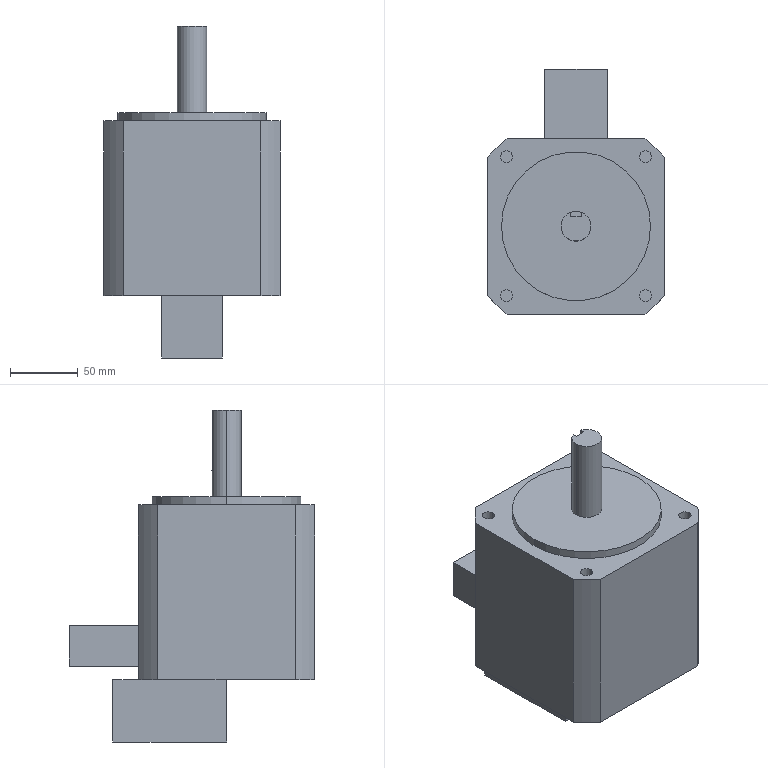Part | SolidWorks | features ICE 7, CirPattern 1, Extrusion 1, HoleWzd 1 | 1 solid | 43 faces | box 130 x 181 x 245 mm | volume 2453559 mm3 | plane 27 | cylinder 16 | commonest cylinder face diameters 9 x8 165 x4 22 x2 110 x2
STEP:
#1=CARTESIAN_POINT('',(46.765,51.265,0.));
#2=VERTEX_POINT('',#1);
#3=CARTESIAN_POINT('',(55.765,51.265,0.));
#4=VERTEX_POINT('',#3);
#5=CARTESIAN_POINT('',(51.265,51.265,0.));
#6=DIRECTION('',(0.,0.,1.));
#7=DIRECTION('',(1.,0.,0.));
#8=AXIS2_PLACEMENT_3D('',#5,#6,#7);
#9=CIRCLE('',#8,4.5);
#10=EDGE_CURVE('',#2,#4,#9,.T.);
#11=ORIENTED_EDGE('',*,*,#10,.F.);
#12=CARTESIAN_POINT('',(46.765,51.265,12.));
#13=VERTEX_POINT('',#12);
#14=CARTESIAN_POINT('',(46.765,51.265,12.));
#15=DIRECTION('',(0.,0.,1.));
#16=VECTOR('',#15,1000.);
#17=LINE('',#14,#16);
#18=EDGE_CURVE('',#2,#13,#17,.T.);
#19=ORIENTED_EDGE('',*,*,#18,.T.);
#20=CARTESIAN_POINT('',(55.765,51.265,12.));
#21=VERTEX_POINT('',#20);
#22=CARTESIAN_POINT('',(51.265,51.265,12.));
#23=DIRECTION('',(0.,0.,1.));
#24=DIRECTION('',(1.,0.,0.));
#25=AXIS2_PLACEMENT_3D('',#22,#23,#24);
#26=CIRCLE('',#25,4.5);
#27=EDGE_CURVE('',#13,#21,#26,.T.);
#28=ORIENTED_EDGE('',*,*,#27,.T.);
#29=CARTESIAN_POINT('',(55.765,51.265,12.));
#30=DIRECTION('',(0.,0.,1.));
#31=VECTOR('',#30,1000.);
#32=LINE('',#29,#31);
#33=EDGE_CURVE('',#4,#21,#32,.T.);
#34=ORIENTED_EDGE('',*,*,#33,.F.);
#35=EDGE_LOOP('',(#11,#19,#28,#34));
#36=FACE_OUTER_BOUND('',#35,.T.);
#37=CARTESIAN_POINT('',(51.265,51.265,12.));
#38=DIRECTION('',(0.,0.,1.));
#39=DIRECTION('',(1.,0.,0.));
#40=AXIS2_PLACEMENT_3D('',#37,#38,#39);
#41=CYLINDRICAL_SURFACE('',#40,4.5);
#42=ADVANCED_FACE('',(#36),#41,.F.);
#43=CARTESIAN_POINT('',(46.765,-51.265,0.));
#44=VERTEX_POINT('',#43);
#45=CARTESIAN_POINT('',(55.765,-51.265,0.));
#46=VERTEX_POINT('',#45);
#47=CARTESIAN_POINT('',(51.265,-51.265,0.));
#48=DIRECTION('',(0.,0.,1.));
#49=DIRECTION('',(1.,0.,0.));
#50=AXIS2_PLACEMENT_3D('',#47,#48,#49);
#51=CIRCLE('',#50,4.5);
#52=EDGE_CURVE('',#44,#46,#51,.T.);
#53=ORIENTED_EDGE('',*,*,#52,.F.);
#54=CARTESIAN_POINT('',(46.765,-51.265,12.));
#55=VERTEX_POINT('',#54);
#56=CARTESIAN_POINT('',(46.765,-51.265,12.));
#57=DIRECTION('',(0.,0.,1.));
#58=VECTOR('',#57,1000.);
#59=LINE('',#56,#58);
#60=EDGE_CURVE('',#44,#55,#59,.T.);
#61=ORIENTED_EDGE('',*,*,#60,.T.);
#62=CARTESIAN_POINT('',(55.765,-51.265,12.));
#63=VERTEX_POINT('',#62);
#64=CARTESIAN_POINT('',(51.265,-51.265,12.));
#65=DIRECTION('',(0.,0.,1.));
#66=DIRECTION('',(1.,0.,0.));
#67=AXIS2_PLACEMENT_3D('',#64,#65,#66);
#68=CIRCLE('',#67,4.5);
#69=EDGE_CURVE('',#55,#63,#68,.T.);
#70=ORIENTED_EDGE('',*,*,#69,.T.);
#71=CARTESIAN_POINT('',(55.765,-51.265,12.));
#72=DIRECTION('',(0.,0.,1.));
#73=VECTOR('',#72,1000.);
#74=LINE('',#71,#73);
#75=EDGE_CURVE('',#46,#63,#74,.T.);
#76=ORIENTED_EDGE('',*,*,#75,.F.);
#77=EDGE_LOOP('',(#53,#61,#70,#76));
#78=FACE_OUTER_BOUND('',#77,.T.);
#79=CARTESIAN_POINT('',(51.265,-51.265,12.));
#80=DIRECTION('',(0.,0.,1.));
#81=DIRECTION('',(1.,0.,0.));
#82=AXIS2_PLACEMENT_3D('',#79,#80,#81);
#83=CYLINDRICAL_SURFACE('',#82,4.5);
#84=ADVANCED_FACE('',(#78),#83,.F.);
#85=CARTESIAN_POINT('',(-55.765,-51.265,0.));
#86=VERTEX_POINT('',#85);
#87=CARTESIAN_POINT('',(-46.765,-51.265,0.));
#88=VERTEX_POINT('',#87);
#89=CARTESIAN_POINT('',(-51.265,-51.265,0.));
#90=DIRECTION('',(0.,0.,1.));
#91=DIRECTION('',(1.,0.,0.));
#92=AXIS2_PLACEMENT_3D('',#89,#90,#91);
#93=CIRCLE('',#92,4.5);
#94=EDGE_CURVE('',#86,#88,#93,.T.);
#95=ORIENTED_EDGE('',*,*,#94,.F.);
#96=CARTESIAN_POINT('',(-55.765,-51.265,12.));
#97=VERTEX_POINT('',#96);
#98=CARTESIAN_POINT('',(-55.765,-51.265,12.));
#99=DIRECTION('',(0.,0.,1.));
#100=VECTOR('',#99,1000.);
#101=LINE('',#98,#100);
#102=EDGE_CURVE('',#86,#97,#101,.T.);
#103=ORIENTED_EDGE('',*,*,#102,.T.);
#104=CARTESIAN_POINT('',(-46.765,-51.265,12.));
#105=VERTEX_POINT('',#104);
#106=CARTESIAN_POINT('',(-51.265,-51.265,12.));
#107=DIRECTION('',(0.,0.,1.));
#108=DIRECTION('',(1.,0.,0.));
#109=AXIS2_PLACEMENT_3D('',#106,#107,#108);
#110=CIRCLE('',#109,4.5);
#111=EDGE_CURVE('',#97,#105,#110,.T.);
#112=ORIENTED_EDGE('',*,*,#111,.T.);
#113=CARTESIAN_POINT('',(-46.765,-51.265,12.));
#114=DIRECTION('',(0.,0.,1.));
#115=VECTOR('',#114,1000.);
#116=LINE('',#113,#115);
#117=EDGE_CURVE('',#88,#105,#116,.T.);
#118=ORIENTED_EDGE('',*,*,#117,.F.);
#119=EDGE_LOOP('',(#95,#103,#112,#118));
#120=FACE_OUTER_BOUND('',#119,.T.);
#121=CARTESIAN_POINT('',(-51.265,-51.265,12.));
#122=DIRECTION('',(0.,0.,1.));
#123=DIRECTION('',(1.,0.,0.));
#124=AXIS2_PLACEMENT_3D('',#121,#122,#123);
#125=CYLINDRICAL_SURFACE('',#124,4.5);
#126=ADVANCED_FACE('',(#120),#125,.F.);
#127=CARTESIAN_POINT('',(-55.765,51.265,0.));
#128=VERTEX_POINT('',#127);
#129=CARTESIAN_POINT('',(-46.765,51.265,0.));
#130=VERTEX_POINT('',#129);
#131=CARTESIAN_POINT('',(-51.265,51.265,0.));
#132=DIRECTION('',(0.,0.,1.));
#133=DIRECTION('',(1.,0.,0.));
#134=AXIS2_PLACEMENT_3D('',#131,#132,#133);
#135=CIRCLE('',#134,4.5);
#136=EDGE_CURVE('',#128,#130,#135,.T.);
#137=ORIENTED_EDGE('',*,*,#136,.F.);
#138=CARTESIAN_POINT('',(-55.765,51.265,12.));
#139=VERTEX_POINT('',#138);
#140=CARTESIAN_POINT('',(-55.765,51.265,12.));
#141=DIRECTION('',(0.,0.,1.));
#142=VECTOR('',#141,1000.);
#143=LINE('',#140,#142);
#144=EDGE_CURVE('',#128,#139,#143,.T.);
#145=ORIENTED_EDGE('',*,*,#144,.T.);
#146=CARTESIAN_POINT('',(-46.765,51.265,12.));
#147=VERTEX_POINT('',#146);
#148=CARTESIAN_POINT('',(-51.265,51.265,12.));
#149=DIRECTION('',(0.,0.,1.));
#150=DIRECTION('',(1.,0.,0.));
#151=AXIS2_PLACEMENT_3D('',#148,#149,#150);
#152=CIRCLE('',#151,4.5);
#153=EDGE_CURVE('',#139,#147,#152,.T.);
#154=ORIENTED_EDGE('',*,*,#153,.T.);
#155=CARTESIAN_POINT('',(-46.765,51.265,12.));
#156=DIRECTION('',(0.,0.,1.));
#157=VECTOR('',#156,1000.);
#158=LINE('',#155,#157);
#159=EDGE_CURVE('',#130,#147,#158,.T.);
#160=ORIENTED_EDGE('',*,*,#159,.F.);
#161=EDGE_LOOP('',(#137,#145,#154,#160));
#162=FACE_OUTER_BOUND('',#161,.T.);
#163=CARTESIAN_POINT('',(-51.265,51.265,12.));
#164=DIRECTION('',(0.,0.,1.));
#165=DIRECTION('',(1.,0.,0.));
#166=AXIS2_PLACEMENT_3D('',#163,#164,#165);
#167=CYLINDRICAL_SURFACE('',#166,4.5);
#168=ADVANCED_FACE('',(#162),#167,.F.);
#169=CARTESIAN_POINT('',(11.,0.,82.));
#170=VERTEX_POINT('',#169);
#171=CARTESIAN_POINT('',(4.,10.247,82.));
#172=VERTEX_POINT('',#171);
#173=CARTESIAN_POINT('',(0.,0.,82.));
#174=DIRECTION('',(0.,0.,1.));
#175=DIRECTION('',(1.,0.,0.));
#176=AXIS2_PLACEMENT_3D('',#173,#174,#175);
#177=CIRCLE('',#176,11.);
#178=EDGE_CURVE('',#170,#172,#177,.T.);
#179=ORIENTED_EDGE('',*,*,#178,.F.);
#180=CARTESIAN_POINT('',(11.,0.,18.));
#181=VERTEX_POINT('',#180);
#182=CARTESIAN_POINT('',(11.,0.,82.));
#183=DIRECTION('',(0.,0.,-1.));
#184=VECTOR('',#183,1000.);
#185=LINE('',#182,#184);
#186=EDGE_CURVE('',#170,#181,#185,.T.);
#187=ORIENTED_EDGE('',*,*,#186,.T.);
#188=CARTESIAN_POINT('',(-11.,0.,18.));
#189=VERTEX_POINT('',#188);
#190=CARTESIAN_POINT('',(0.,0.,18.));
#191=DIRECTION('',(0.,0.,1.));
#192=DIRECTION('',(1.,0.,0.));
#193=AXIS2_PLACEMENT_3D('',#190,#191,#192);
#194=CIRCLE('',#193,11.);
#195=EDGE_CURVE('',#181,#189,#194,.T.);
#196=ORIENTED_EDGE('',*,*,#195,.T.);
#197=CARTESIAN_POINT('',(-11.,0.,82.));
#198=VERTEX_POINT('',#197);
#199=CARTESIAN_POINT('',(-11.,0.,82.));
#200=DIRECTION('',(0.,0.,-1.));
#201=VECTOR('',#200,1000.);
#202=LINE('',#199,#201);
#203=EDGE_CURVE('',#198,#189,#202,.T.);
#204=ORIENTED_EDGE('',*,*,#203,.F.);
#205=CARTESIAN_POINT('',(-4.,10.247,82.));
#206=VERTEX_POINT('',#205);
#207=CARTESIAN_POINT('',(0.,0.,82.));
#208=DIRECTION('',(0.,0.,1.));
#209=DIRECTION('',(1.,0.,0.));
#210=AXIS2_PLACEMENT_3D('',#207,#208,#209);
#211=CIRCLE('',#210,11.);
#212=EDGE_CURVE('',#206,#198,#211,.T.);
#213=ORIENTED_EDGE('',*,*,#212,.F.);
#214=CARTESIAN_POINT('',(-4.,10.247,37.));
#215=VERTEX_POINT('',#214);
#216=CARTESIAN_POINT('',(-4.,10.247,82.));
#217=DIRECTION('',(0.,0.,-1.));
#218=VECTOR('',#217,1000.);
#219=LINE('',#216,#218);
#220=EDGE_CURVE('',#206,#215,#219,.T.);
#221=ORIENTED_EDGE('',*,*,#220,.T.);
#222=CARTESIAN_POINT('',(4.,10.247,37.));
#223=VERTEX_POINT('',#222);
#224=CARTESIAN_POINT('',(0.,0.,37.));
#225=DIRECTION('',(0.,0.,-1.));
#226=DIRECTION('',(-1.,0.,0.));
#227=AXIS2_PLACEMENT_3D('',#224,#225,#226);
#228=CIRCLE('',#227,11.);
#229=EDGE_CURVE('',#215,#223,#228,.T.);
#230=ORIENTED_EDGE('',*,*,#229,.T.);
#231=CARTESIAN_POINT('',(4.,10.247,82.));
#232=DIRECTION('',(0.,0.,1.));
#233=VECTOR('',#232,1000.);
#234=LINE('',#231,#233);
#235=EDGE_CURVE('',#223,#172,#234,.T.);
#236=ORIENTED_EDGE('',*,*,#235,.T.);
#237=EDGE_LOOP('',(#179,#187,#196,#204,#213,#221,#230,#236));
#238=FACE_OUTER_BOUND('',#237,.T.);
#239=CARTESIAN_POINT('',(0.,0.,82.));
#240=DIRECTION('',(0.,0.,-1.));
#241=DIRECTION('',(-1.,0.,0.));
#242=AXIS2_PLACEMENT_3D('',#239,#240,#241);
#243=CYLINDRICAL_SURFACE('',#242,11.);
#244=ADVANCED_FACE('',(#238),#243,.T.);
#245=CARTESIAN_POINT('',(55.,0.,18.));
#246=VERTEX_POINT('',#245);
#247=CARTESIAN_POINT('',(-55.,0.,18.));
#248=VERTEX_POINT('',#247);
#249=CARTESIAN_POINT('',(0.,0.,18.));
#250=DIRECTION('',(0.,0.,1.));
#251=DIRECTION('',(1.,0.,0.));
#252=AXIS2_PLACEMENT_3D('',#249,#250,#251);
#253=CIRCLE('',#252,55.);
#254=EDGE_CURVE('',#246,#248,#253,.T.);
#255=ORIENTED_EDGE('',*,*,#254,.F.);
#256=CARTESIAN_POINT('',(55.,0.,12.));
#257=VERTEX_POINT('',#256);
#258=CARTESIAN_POINT('',(55.,0.,18.));
#259=DIRECTION('',(0.,0.,-1.));
#260=VECTOR('',#259,1000.);
#261=LINE('',#258,#260);
#262=EDGE_CURVE('',#246,#257,#261,.T.);
#263=ORIENTED_EDGE('',*,*,#262,.T.);
#264=CARTESIAN_POINT('',(-55.,0.,12.));
#265=VERTEX_POINT('',#264);
#266=CARTESIAN_POINT('',(0.,0.,12.));
#267=DIRECTION('',(0.,0.,1.));
#268=DIRECTION('',(1.,0.,0.));
#269=AXIS2_PLACEMENT_3D('',#266,#267,#268);
#270=CIRCLE('',#269,55.);
#271=EDGE_CURVE('',#257,#265,#270,.T.);
#272=ORIENTED_EDGE('',*,*,#271,.T.);
#273=CARTESIAN_POINT('',(-55.,0.,18.));
#274=DIRECTION('',(0.,0.,-1.));
#275=VECTOR('',#274,1000.);
#276=LINE('',#273,#275);
#277=EDGE_CURVE('',#248,#265,#276,.T.);
#278=ORIENTED_EDGE('',*,*,#277,.F.);
#279=EDGE_LOOP('',(#255,#263,#272,#278));
#280=FACE_OUTER_BOUND('',#279,.T.);
#281=CARTESIAN_POINT('',(0.,0.,18.));
#282=DIRECTION('',(0.,0.,-1.));
#283=DIRECTION('',(-1.,0.,0.));
#284=AXIS2_PLACEMENT_3D('',#281,#282,#283);
#285=CYLINDRICAL_SURFACE('',#284,55.);
#286=ADVANCED_FACE('',(#280),#285,.T.);
#287=CARTESIAN_POINT('',(51.265,51.265,12.));
#288=DIRECTION('',(0.,0.,1.));
#289=DIRECTION('',(1.,0.,0.));
#290=AXIS2_PLACEMENT_3D('',#287,#288,#289);
#291=CIRCLE('',#290,4.5);
#292=EDGE_CURVE('',#21,#13,#291,.T.);
#293=ORIENTED_EDGE('',*,*,#292,.F.);
#294=ORIENTED_EDGE('',*,*,#27,.F.);
#295=EDGE_LOOP('',(#293,#294));
#296=FACE_BOUND('',#295,.T.);
#297=CARTESIAN_POINT('',(51.265,-51.265,12.));
#298=DIRECTION('',(0.,0.,1.));
#299=DIRECTION('',(1.,0.,0.));
#300=AXIS2_PLACEMENT_3D('',#297,#298,#299);
#301=CIRCLE('',#300,4.5);
#302=EDGE_CURVE('',#63,#55,#301,.T.);
#303=ORIENTED_EDGE('',*,*,#302,.F.);
#304=ORIENTED_EDGE('',*,*,#69,.F.);
#305=EDGE_LOOP('',(#303,#304));
#306=FACE_BOUND('',#305,.T.);
#307=CARTESIAN_POINT('',(-51.265,-51.265,12.));
#308=DIRECTION('',(0.,0.,1.));
#309=DIRECTION('',(1.,0.,0.));
#310=AXIS2_PLACEMENT_3D('',#307,#308,#309);
#311=CIRCLE('',#310,4.5);
#312=EDGE_CURVE('',#105,#97,#311,.T.);
#313=ORIENTED_EDGE('',*,*,#312,.F.);
#314=ORIENTED_EDGE('',*,*,#111,.F.);
#315=EDGE_LOOP('',(#313,#314));
#316=FACE_BOUND('',#315,.T.);
#317=CARTESIAN_POINT('',(-51.265,51.265,12.));
#318=DIRECTION('',(0.,0.,1.));
#319=DIRECTION('',(1.,0.,0.));
#320=AXIS2_PLACEMENT_3D('',#317,#318,#319);
#321=CIRCLE('',#320,4.5);
#322=EDGE_CURVE('',#147,#139,#321,.T.);
#323=ORIENTED_EDGE('',*,*,#322,.F.);
#324=ORIENTED_EDGE('',*,*,#153,.F.);
#325=EDGE_LOOP('',(#323,#324));
#326=FACE_BOUND('',#325,.T.);
#327=CARTESIAN_POINT('',(0.,0.,12.));
#328=DIRECTION('',(0.,0.,1.));
#329=DIRECTION('',(1.,0.,0.));
#330=AXIS2_PLACEMENT_3D('',#327,#328,#329);
#331=CIRCLE('',#330,55.);
#332=EDGE_CURVE('',#265,#257,#331,.T.);
#333=ORIENTED_EDGE('',*,*,#332,.F.);
#334=ORIENTED_EDGE('',*,*,#271,.F.);
#335=EDGE_LOOP('',(#333,#334));
#336=FACE_BOUND('',#335,.T.);
#337=CARTESIAN_POINT('',(65.,-50.806,12.));
#338=VERTEX_POINT('',#337);
#339=CARTESIAN_POINT('',(65.,50.806,12.));
#340=VERTEX_POINT('',#339);
#341=CARTESIAN_POINT('',(65.,65.,12.));
#342=DIRECTION('',(0.,1.,0.));
#343=VECTOR('',#342,1000.);
#344=LINE('',#341,#343);
#345=EDGE_CURVE('',#338,#340,#344,.T.);
#346=ORIENTED_EDGE('',*,*,#345,.T.);
#347=CARTESIAN_POINT('',(50.806,65.,12.));
#348=VERTEX_POINT('',#347);
#349=CARTESIAN_POINT('',(0.,0.,12.));
#350=DIRECTION('',(0.,0.,1.));
#351=DIRECTION('',(1.,0.,0.));
#352=AXIS2_PLACEMENT_3D('',#349,#350,#351);
#353=CIRCLE('',#352,82.5);
#354=EDGE_CURVE('',#340,#348,#353,.T.);
#355=ORIENTED_EDGE('',*,*,#354,.T.);
#356=CARTESIAN_POINT('',(-50.806,65.,12.));
#357=VERTEX_POINT('',#356);
#358=CARTESIAN_POINT('',(-65.,65.,12.));
#359=DIRECTION('',(-1.,0.,0.));
#360=VECTOR('',#359,1000.);
#361=LINE('',#358,#360);
#362=EDGE_CURVE('',#348,#357,#361,.T.);
#363=ORIENTED_EDGE('',*,*,#362,.T.);
#364=CARTESIAN_POINT('',(-65.,50.806,12.));
#365=VERTEX_POINT('',#364);
#366=CARTESIAN_POINT('',(0.,0.,12.));
#367=DIRECTION('',(0.,0.,1.));
#368=DIRECTION('',(1.,0.,0.));
#369=AXIS2_PLACEMENT_3D('',#366,#367,#368);
#370=CIRCLE('',#369,82.5);
#371=EDGE_CURVE('',#357,#365,#370,.T.);
#372=ORIENTED_EDGE('',*,*,#371,.T.);
#373=CARTESIAN_POINT('',(-65.,-50.806,12.));
#374=VERTEX_POINT('',#373);
#375=CARTESIAN_POINT('',(-65.,65.,12.));
#376=DIRECTION('',(0.,-1.,0.));
#377=VECTOR('',#376,1000.);
#378=LINE('',#375,#377);
#379=EDGE_CURVE('',#365,#374,#378,.T.);
#380=ORIENTED_EDGE('',*,*,#379,.T.);
#381=CARTESIAN_POINT('',(-50.806,-65.,12.));
#382=VERTEX_POINT('',#381);
#383=CARTESIAN_POINT('',(0.,0.,12.));
#384=DIRECTION('',(0.,0.,1.));
#385=DIRECTION('',(1.,0.,0.));
#386=AXIS2_PLACEMENT_3D('',#383,#384,#385);
#387=CIRCLE('',#386,82.5);
#388=EDGE_CURVE('',#374,#382,#387,.T.);
#389=ORIENTED_EDGE('',*,*,#388,.T.);
#390=CARTESIAN_POINT('',(50.806,-65.,12.));
#391=VERTEX_POINT('',#390);
#392=CARTESIAN_POINT('',(-65.,-65.,12.));
#393=DIRECTION('',(1.,0.,0.));
#394=VECTOR('',#393,1000.);
#395=LINE('',#392,#394);
#396=EDGE_CURVE('',#382,#391,#395,.T.);
#397=ORIENTED_EDGE('',*,*,#396,.T.);
#398=CARTESIAN_POINT('',(0.,0.,12.));
#399=DIRECTION('',(0.,0.,1.));
#400=DIRECTION('',(1.,0.,0.));
#401=AXIS2_PLACEMENT_3D('',#398,#399,#400);
#402=CIRCLE('',#401,82.5);
#403=EDGE_CURVE('',#391,#338,#402,.T.);
#404=ORIENTED_EDGE('',*,*,#403,.T.);
#405=EDGE_LOOP('',(#346,#355,#363,#372,#380,#389,#397,#404));
#406=FACE_OUTER_BOUND('',#405,.T.);
#407=CARTESIAN_POINT('',(65.,-65.,12.));
#408=DIRECTION('',(0.,0.,1.));
#409=DIRECTION('',(1.,0.,0.));
#410=AXIS2_PLACEMENT_3D('',#407,#408,#409);
#411=PLANE('',#410);
#412=ADVANCED_FACE('',(#296,#306,#316,#326,#336,#406),#411,.T.);
#413=CARTESIAN_POINT('',(65.,-50.806,-117.));
#414=VERTEX_POINT('',#413);
#415=CARTESIAN_POINT('',(65.,-50.806,-52.));
#416=DIRECTION('',(0.,0.,1.));
#417=VECTOR('',#416,1000.);
#418=LINE('',#415,#417);
#419=EDGE_CURVE('',#414,#338,#418,.T.);
#420=ORIENTED_EDGE('',*,*,#419,.F.);
#421=CARTESIAN_POINT('',(65.,50.806,-117.));
#422=VERTEX_POINT('',#421);
#423=CARTESIAN_POINT('',(65.,50.806,-117.));
#424=DIRECTION('',(0.,-1.,0.));
#425=VECTOR('',#424,1000.);
#426=LINE('',#423,#425);
#427=EDGE_CURVE('',#422,#414,#426,.T.);
#428=ORIENTED_EDGE('',*,*,#427,.F.);
#429=CARTESIAN_POINT('',(65.,50.806,-52.));
#430=DIRECTION('',(0.,0.,-1.));
#431=VECTOR('',#430,1000.);
#432=LINE('',#429,#431);
#433=EDGE_CURVE('',#340,#422,#432,.T.);
#434=ORIENTED_EDGE('',*,*,#433,.F.);
#435=ORIENTED_EDGE('',*,*,#345,.F.);
#436=EDGE_LOOP('',(#420,#428,#434,#435));
#437=FACE_OUTER_BOUND('',#436,.T.);
#438=CARTESIAN_POINT('',(65.,65.,12.));
#439=DIRECTION('',(-1.,0.,0.));
#440=DIRECTION('',(0.,-1.,0.));
#441=AXIS2_PLACEMENT_3D('',#438,#439,#440);
#442=PLANE('',#441);
#443=ADVANCED_FACE('',(#437),#442,.F.);
#444=CARTESIAN_POINT('',(23.,65.,-107.));
#445=VERTEX_POINT('',#444);
#446=CARTESIAN_POINT('',(-23.,65.,-107.));
#447=VERTEX_POINT('',#446);
#448=CARTESIAN_POINT('',(23.,65.,-107.));
#449=DIRECTION('',(-1.,0.,0.));
#450=VECTOR('',#449,1000.);
#451=LINE('',#448,#450);
#452=EDGE_CURVE('',#445,#447,#451,.T.);
#453=ORIENTED_EDGE('',*,*,#452,.F.);
#454=CARTESIAN_POINT('',(23.,65.,-77.));
#455=VERTEX_POINT('',#454);
#456=CARTESIAN_POINT('',(23.,65.,-107.));
#457=DIRECTION('',(0.,0.,-1.));
#458=VECTOR('',#457,1000.);
#459=LINE('',#456,#458);
#460=EDGE_CURVE('',#455,#445,#459,.T.);
#461=ORIENTED_EDGE('',*,*,#460,.F.);
#462=CARTESIAN_POINT('',(-23.,65.,-77.));
#463=VERTEX_POINT('',#462);
#464=CARTESIAN_POINT('',(23.,65.,-77.));
#465=DIRECTION('',(-1.,0.,0.));
#466=VECTOR('',#465,1000.);
#467=LINE('',#464,#466);
#468=EDGE_CURVE('',#455,#463,#467,.T.);
#469=ORIENTED_EDGE('',*,*,#468,.T.);
#470=CARTESIAN_POINT('',(-23.,65.,-107.));
#471=DIRECTION('',(0.,0.,-1.));
#472=VECTOR('',#471,1000.);
#473=LINE('',#470,#472);
#474=EDGE_CURVE('',#463,#447,#473,.T.);
#475=ORIENTED_EDGE('',*,*,#474,.T.);
#476=EDGE_LOOP('',(#453,#461,#469,#475));
#477=FACE_BOUND('',#476,.T.);
#478=CARTESIAN_POINT('',(50.806,65.,-117.));
#479=VERTEX_POINT('',#478);
#480=CARTESIAN_POINT('',(50.806,65.,-52.));
#481=DIRECTION('',(0.,0.,1.));
#482=VECTOR('',#481,1000.);
#483=LINE('',#480,#482);
#484=EDGE_CURVE('',#479,#348,#483,.T.);
#485=ORIENTED_EDGE('',*,*,#484,.F.);
#486=CARTESIAN_POINT('',(22.5,65.,-117.));
#487=VERTEX_POINT('',#486);
#488=CARTESIAN_POINT('',(-50.806,65.,-117.));
#489=DIRECTION('',(1.,0.,0.));
#490=VECTOR('',#489,1000.);
#491=LINE('',#488,#490);
#492=EDGE_CURVE('',#487,#479,#491,.T.);
#493=ORIENTED_EDGE('',*,*,#492,.F.);
#494=CARTESIAN_POINT('',(-22.5,65.,-117.));
#495=VERTEX_POINT('',#494);
#496=CARTESIAN_POINT('',(-50.806,65.,-117.));
#497=DIRECTION('',(1.,0.,0.));
#498=VECTOR('',#497,1000.);
#499=LINE('',#496,#498);
#500=EDGE_CURVE('',#495,#487,#499,.T.);
#501=ORIENTED_EDGE('',*,*,#500,.F.);
#502=CARTESIAN_POINT('',(-50.806,65.,-117.));
#503=VERTEX_POINT('',#502);
#504=CARTESIAN_POINT('',(-50.806,65.,-117.));
#505=DIRECTION('',(1.,0.,0.));
#506=VECTOR('',#505,1000.);
#507=LINE('',#504,#506);
#508=EDGE_CURVE('',#503,#495,#507,.T.);
#509=ORIENTED_EDGE('',*,*,#508,.F.);
#510=CARTESIAN_POINT('',(-50.806,65.,-52.));
#511=DIRECTION('',(0.,0.,-1.));
#512=VECTOR('',#511,1000.);
#513=LINE('',#510,#512);
#514=EDGE_CURVE('',#357,#503,#513,.T.);
#515=ORIENTED_EDGE('',*,*,#514,.F.);
#516=ORIENTED_EDGE('',*,*,#362,.F.);
#517=EDGE_LOOP('',(#485,#493,#501,#509,#515,#516));
#518=FACE_OUTER_BOUND('',#517,.T.);
#519=CARTESIAN_POINT('',(-65.,65.,12.));
#520=DIRECTION('',(0.,-1.,0.));
#521=DIRECTION('',(0.,0.,-1.));
#522=AXIS2_PLACEMENT_3D('',#519,#520,#521);
#523=PLANE('',#522);
#524=ADVANCED_FACE('',(#477,#518),#523,.F.);
#525=CARTESIAN_POINT('',(-65.,50.806,-117.));
#526=VERTEX_POINT('',#525);
#527=CARTESIAN_POINT('',(-65.,50.806,-52.));
#528=DIRECTION('',(0.,0.,1.));
#529=VECTOR('',#528,1000.);
#530=LINE('',#527,#529);
#531=EDGE_CURVE('',#526,#365,#530,.T.);
#532=ORIENTED_EDGE('',*,*,#531,.F.);
#533=CARTESIAN_POINT('',(-65.,-50.806,-117.));
#534=VERTEX_POINT('',#533);
#535=CARTESIAN_POINT('',(-65.,-50.806,-117.));
#536=DIRECTION('',(0.,1.,0.));
#537=VECTOR('',#536,1000.);
#538=LINE('',#535,#537);
#539=EDGE_CURVE('',#534,#526,#538,.T.);
#540=ORIENTED_EDGE('',*,*,#539,.F.);
#541=CARTESIAN_POINT('',(-65.,-50.806,-52.));
#542=DIRECTION('',(0.,0.,-1.));
#543=VECTOR('',#542,1000.);
#544=LINE('',#541,#543);
#545=EDGE_CURVE('',#374,#534,#544,.T.);
#546=ORIENTED_EDGE('',*,*,#545,.F.);
#547=ORIENTED_EDGE('',*,*,#379,.F.);
#548=EDGE_LOOP('',(#532,#540,#546,#547));
#549=FACE_OUTER_BOUND('',#548,.T.);
#550=CARTESIAN_POINT('',(-65.,65.,12.));
#551=DIRECTION('',(1.,0.,0.));
#552=DIRECTION('',(0.,1.,0.));
#553=AXIS2_PLACEMENT_3D('',#550,#551,#552);
#554=PLANE('',#553);
#555=ADVANCED_FACE('',(#549),#554,.F.);
#556=CARTESIAN_POINT('',(-50.806,-65.,-117.));
#557=VERTEX_POINT('',#556);
#558=CARTESIAN_POINT('',(-50.806,-65.,-52.));
#559=DIRECTION('',(0.,0.,1.));
#560=VECTOR('',#559,1000.);
#561=LINE('',#558,#560);
#562=EDGE_CURVE('',#557,#382,#561,.T.);
#563=ORIENTED_EDGE('',*,*,#562,.F.);
#564=CARTESIAN_POINT('',(50.806,-65.,-117.));
#565=VERTEX_POINT('',#564);
#566=CARTESIAN_POINT('',(50.806,-65.,-117.));
#567=DIRECTION('',(-1.,0.,0.));
#568=VECTOR('',#567,1000.);
#569=LINE('',#566,#568);
#570=EDGE_CURVE('',#565,#557,#569,.T.);
#571=ORIENTED_EDGE('',*,*,#570,.F.);
#572=CARTESIAN_POINT('',(50.806,-65.,-52.));
#573=DIRECTION('',(0.,0.,-1.));
#574=VECTOR('',#573,1000.);
#575=LINE('',#572,#574);
#576=EDGE_CURVE('',#391,#565,#575,.T.);
#577=ORIENTED_EDGE('',*,*,#576,.F.);
#578=ORIENTED_EDGE('',*,*,#396,.F.);
#579=EDGE_LOOP('',(#563,#571,#577,#578));
#580=FACE_OUTER_BOUND('',#579,.T.);
#581=CARTESIAN_POINT('',(-65.,-65.,12.));
#582=DIRECTION('',(0.,1.,0.));
#583=DIRECTION('',(0.,0.,1.));
#584=AXIS2_PLACEMENT_3D('',#581,#582,#583);
#585=PLANE('',#584);
#586=ADVANCED_FACE('',(#580),#585,.F.);
#587=CARTESIAN_POINT('',(0.,0.,18.));
#588=DIRECTION('',(0.,0.,1.));
#589=DIRECTION('',(1.,0.,0.));
#590=AXIS2_PLACEMENT_3D('',#587,#588,#589);
#591=CIRCLE('',#590,55.);
#592=EDGE_CURVE('',#248,#246,#591,.T.);
#593=ORIENTED_EDGE('',*,*,#592,.T.);
#594=ORIENTED_EDGE('',*,*,#254,.T.);
#595=EDGE_LOOP('',(#593,#594));
#596=FACE_OUTER_BOUND('',#595,.T.);
#597=CARTESIAN_POINT('',(0.,0.,18.));
#598=DIRECTION('',(0.,0.,1.));
#599=DIRECTION('',(1.,0.,0.));
#600=AXIS2_PLACEMENT_3D('',#597,#598,#599);
#601=CIRCLE('',#600,11.);
#602=EDGE_CURVE('',#189,#181,#601,.T.);
#603=ORIENTED_EDGE('',*,*,#602,.F.);
#604=ORIENTED_EDGE('',*,*,#195,.F.);
#605=EDGE_LOOP('',(#603,#604));
#606=FACE_BOUND('',#605,.T.);
#607=CARTESIAN_POINT('',(0.,0.,18.));
#608=DIRECTION('',(0.,0.,1.));
#609=DIRECTION('',(1.,0.,0.));
#610=AXIS2_PLACEMENT_3D('',#607,#608,#609);
#611=PLANE('',#610);
#612=ADVANCED_FACE('',(#596,#606),#611,.T.);
#613=ORIENTED_EDGE('',*,*,#262,.F.);
#614=ORIENTED_EDGE('',*,*,#592,.F.);
#615=ORIENTED_EDGE('',*,*,#277,.T.);
#616=ORIENTED_EDGE('',*,*,#332,.T.);
#617=EDGE_LOOP('',(#613,#614,#615,#616));
#618=FACE_OUTER_BOUND('',#617,.T.);
#619=CARTESIAN_POINT('',(0.,0.,18.));
#620=DIRECTION('',(0.,0.,-1.));
#621=DIRECTION('',(-1.,0.,0.));
#622=AXIS2_PLACEMENT_3D('',#619,#620,#621);
#623=CYLINDRICAL_SURFACE('',#622,55.);
#624=ADVANCED_FACE('',(#618),#623,.T.);
#625=ORIENTED_EDGE('',*,*,#186,.F.);
#626=CARTESIAN_POINT('',(0.,0.,82.));
#627=DIRECTION('',(0.,0.,1.));
#628=DIRECTION('',(1.,0.,0.));
#629=AXIS2_PLACEMENT_3D('',#626,#627,#628);
#630=CIRCLE('',#629,11.);
#631=EDGE_CURVE('',#198,#170,#630,.T.);
#632=ORIENTED_EDGE('',*,*,#631,.F.);
#633=ORIENTED_EDGE('',*,*,#203,.T.);
#634=ORIENTED_EDGE('',*,*,#602,.T.);
#635=EDGE_LOOP('',(#625,#632,#633,#634));
#636=FACE_OUTER_BOUND('',#635,.T.);
#637=CARTESIAN_POINT('',(0.,0.,82.));
#638=DIRECTION('',(0.,0.,-1.));
#639=DIRECTION('',(-1.,0.,0.));
#640=AXIS2_PLACEMENT_3D('',#637,#638,#639);
#641=CYLINDRICAL_SURFACE('',#640,11.);
#642=ADVANCED_FACE('',(#636),#641,.T.);
#643=CARTESIAN_POINT('',(4.,7.,82.));
#644=VERTEX_POINT('',#643);
#645=CARTESIAN_POINT('',(4.,7.,82.));
#646=DIRECTION('',(0.,1.,0.));
#647=VECTOR('',#646,1000.);
#648=LINE('',#645,#647);
#649=EDGE_CURVE('',#644,#172,#648,.T.);
#650=ORIENTED_EDGE('',*,*,#649,.F.);
#651=CARTESIAN_POINT('',(-4.,7.,82.));
#652=VERTEX_POINT('',#651);
#653=CARTESIAN_POINT('',(-4.,7.,82.));
#654=DIRECTION('',(1.,0.,0.));
#655=VECTOR('',#654,1000.);
#656=LINE('',#653,#655);
#657=EDGE_CURVE('',#652,#644,#656,.T.);
#658=ORIENTED_EDGE('',*,*,#657,.F.);
#659=CARTESIAN_POINT('',(-4.,0.,82.));
#660=DIRECTION('',(0.,-1.,0.));
#661=VECTOR('',#660,1000.);
#662=LINE('',#659,#661);
#663=EDGE_CURVE('',#206,#652,#662,.T.);
#664=ORIENTED_EDGE('',*,*,#663,.F.);
#665=ORIENTED_EDGE('',*,*,#212,.T.);
#666=ORIENTED_EDGE('',*,*,#631,.T.);
#667=ORIENTED_EDGE('',*,*,#178,.T.);
#668=EDGE_LOOP('',(#650,#658,#664,#665,#666,#667));
#669=FACE_OUTER_BOUND('',#668,.T.);
#670=CARTESIAN_POINT('',(0.,0.,82.));
#671=DIRECTION('',(0.,0.,1.));
#672=DIRECTION('',(1.,0.,0.));
#673=AXIS2_PLACEMENT_3D('',#670,#671,#672);
#674=PLANE('',#673);
#675=ADVANCED_FACE('',(#669),#674,.T.);
#676=ORIENTED_EDGE('',*,*,#419,.T.);
#677=ORIENTED_EDGE('',*,*,#403,.F.);
#678=ORIENTED_EDGE('',*,*,#576,.T.);
#679=CARTESIAN_POINT('',(0.,0.,-117.));
#680=DIRECTION('',(0.,0.,-1.));
#681=DIRECTION('',(-1.,0.,0.));
#682=AXIS2_PLACEMENT_3D('',#679,#680,#681);
#683=CIRCLE('',#682,82.5);
#684=EDGE_CURVE('',#414,#565,#683,.T.);
#685=ORIENTED_EDGE('',*,*,#684,.F.);
#686=EDGE_LOOP('',(#676,#677,#678,#685));
#687=FACE_OUTER_BOUND('',#686,.T.);
#688=CARTESIAN_POINT('',(0.,0.,-52.));
#689=DIRECTION('',(0.,0.,1.));
#690=DIRECTION('',(1.,0.,0.));
#691=AXIS2_PLACEMENT_3D('',#688,#689,#690);
#692=CYLINDRICAL_SURFACE('',#691,82.5);
#693=ADVANCED_FACE('',(#687),#692,.T.);
#694=ORIENTED_EDGE('',*,*,#545,.T.);
#695=CARTESIAN_POINT('',(0.,0.,-117.));
#696=DIRECTION('',(0.,0.,-1.));
#697=DIRECTION('',(-1.,0.,0.));
#698=AXIS2_PLACEMENT_3D('',#695,#696,#697);
#699=CIRCLE('',#698,82.5);
#700=EDGE_CURVE('',#557,#534,#699,.T.);
#701=ORIENTED_EDGE('',*,*,#700,.F.);
#702=ORIENTED_EDGE('',*,*,#562,.T.);
#703=ORIENTED_EDGE('',*,*,#388,.F.);
#704=EDGE_LOOP('',(#694,#701,#702,#703));
#705=FACE_OUTER_BOUND('',#704,.T.);
#706=CARTESIAN_POINT('',(0.,0.,-52.));
#707=DIRECTION('',(0.,0.,1.));
#708=DIRECTION('',(1.,0.,0.));
#709=AXIS2_PLACEMENT_3D('',#706,#707,#708);
#710=CYLINDRICAL_SURFACE('',#709,82.5);
#711=ADVANCED_FACE('',(#705),#710,.T.);
#712=ORIENTED_EDGE('',*,*,#514,.T.);
#713=CARTESIAN_POINT('',(0.,0.,-117.));
#714=DIRECTION('',(0.,0.,-1.));
#715=DIRECTION('',(-1.,0.,0.));
#716=AXIS2_PLACEMENT_3D('',#713,#714,#715);
#717=CIRCLE('',#716,82.5);
#718=EDGE_CURVE('',#526,#503,#717,.T.);
#719=ORIENTED_EDGE('',*,*,#718,.F.);
#720=ORIENTED_EDGE('',*,*,#531,.T.);
#721=ORIENTED_EDGE('',*,*,#371,.F.);
#722=EDGE_LOOP('',(#712,#719,#720,#721));
#723=FACE_OUTER_BOUND('',#722,.T.);
#724=CARTESIAN_POINT('',(0.,0.,-52.));
#725=DIRECTION('',(0.,0.,1.));
#726=DIRECTION('',(1.,0.,0.));
#727=AXIS2_PLACEMENT_3D('',#724,#725,#726);
#728=CYLINDRICAL_SURFACE('',#727,82.5);
#729=ADVANCED_FACE('',(#723),#728,.T.);
#730=ORIENTED_EDGE('',*,*,#433,.T.);
#731=CARTESIAN_POINT('',(0.,0.,-117.));
#732=DIRECTION('',(0.,0.,-1.));
#733=DIRECTION('',(-1.,0.,0.));
#734=AXIS2_PLACEMENT_3D('',#731,#732,#733);
#735=CIRCLE('',#734,82.5);
#736=EDGE_CURVE('',#479,#422,#735,.T.);
#737=ORIENTED_EDGE('',*,*,#736,.F.);
#738=ORIENTED_EDGE('',*,*,#484,.T.);
#739=ORIENTED_EDGE('',*,*,#354,.F.);
#740=EDGE_LOOP('',(#730,#737,#738,#739));
#741=FACE_OUTER_BOUND('',#740,.T.);
#742=CARTESIAN_POINT('',(0.,0.,-52.));
#743=DIRECTION('',(0.,0.,1.));
#744=DIRECTION('',(1.,0.,0.));
#745=AXIS2_PLACEMENT_3D('',#742,#743,#744);
#746=CYLINDRICAL_SURFACE('',#745,82.5);
#747=ADVANCED_FACE('',(#741),#746,.T.);
#748=ORIENTED_EDGE('',*,*,#144,.F.);
#749=CARTESIAN_POINT('',(-51.265,51.265,0.));
#750=DIRECTION('',(0.,0.,1.));
#751=DIRECTION('',(1.,0.,0.));
#752=AXIS2_PLACEMENT_3D('',#749,#750,#751);
#753=CIRCLE('',#752,4.5);
#754=EDGE_CURVE('',#130,#128,#753,.T.);
#755=ORIENTED_EDGE('',*,*,#754,.F.);
#756=ORIENTED_EDGE('',*,*,#159,.T.);
#757=ORIENTED_EDGE('',*,*,#322,.T.);
#758=EDGE_LOOP('',(#748,#755,#756,#757));
#759=FACE_OUTER_BOUND('',#758,.T.);
#760=CARTESIAN_POINT('',(-51.265,51.265,12.));
#761=DIRECTION('',(0.,0.,1.));
#762=DIRECTION('',(1.,0.,0.));
#763=AXIS2_PLACEMENT_3D('',#760,#761,#762);
#764=CYLINDRICAL_SURFACE('',#763,4.5);
#765=ADVANCED_FACE('',(#759),#764,.F.);
#766=ORIENTED_EDGE('',*,*,#102,.F.);
#767=CARTESIAN_POINT('',(-51.265,-51.265,0.));
#768=DIRECTION('',(0.,0.,1.));
#769=DIRECTION('',(1.,0.,0.));
#770=AXIS2_PLACEMENT_3D('',#767,#768,#769);
#771=CIRCLE('',#770,4.5);
#772=EDGE_CURVE('',#88,#86,#771,.T.);
#773=ORIENTED_EDGE('',*,*,#772,.F.);
#774=ORIENTED_EDGE('',*,*,#117,.T.);
#775=ORIENTED_EDGE('',*,*,#312,.T.);
#776=EDGE_LOOP('',(#766,#773,#774,#775));
#777=FACE_OUTER_BOUND('',#776,.T.);
#778=CARTESIAN_POINT('',(-51.265,-51.265,12.));
#779=DIRECTION('',(0.,0.,1.));
#780=DIRECTION('',(1.,0.,0.));
#781=AXIS2_PLACEMENT_3D('',#778,#779,#780);
#782=CYLINDRICAL_SURFACE('',#781,4.5);
#783=ADVANCED_FACE('',(#777),#782,.F.);
#784=ORIENTED_EDGE('',*,*,#60,.F.);
#785=CARTESIAN_POINT('',(51.265,-51.265,0.));
#786=DIRECTION('',(0.,0.,1.));
#787=DIRECTION('',(1.,0.,0.));
#788=AXIS2_PLACEMENT_3D('',#785,#786,#787);
#789=CIRCLE('',#788,4.5);
#790=EDGE_CURVE('',#46,#44,#789,.T.);
#791=ORIENTED_EDGE('',*,*,#790,.F.);
#792=ORIENTED_EDGE('',*,*,#75,.T.);
#793=ORIENTED_EDGE('',*,*,#302,.T.);
#794=EDGE_LOOP('',(#784,#791,#792,#793));
#795=FACE_OUTER_BOUND('',#794,.T.);
#796=CARTESIAN_POINT('',(51.265,-51.265,12.));
#797=DIRECTION('',(0.,0.,1.));
#798=DIRECTION('',(1.,0.,0.));
#799=AXIS2_PLACEMENT_3D('',#796,#797,#798);
#800=CYLINDRICAL_SURFACE('',#799,4.5);
#801=ADVANCED_FACE('',(#795),#800,.F.);
#802=ORIENTED_EDGE('',*,*,#18,.F.);
#803=CARTESIAN_POINT('',(51.265,51.265,0.));
#804=DIRECTION('',(0.,0.,1.));
#805=DIRECTION('',(1.,0.,0.));
#806=AXIS2_PLACEMENT_3D('',#803,#804,#805);
#807=CIRCLE('',#806,4.5);
#808=EDGE_CURVE('',#4,#2,#807,.T.);
#809=ORIENTED_EDGE('',*,*,#808,.F.);
#810=ORIENTED_EDGE('',*,*,#33,.T.);
#811=ORIENTED_EDGE('',*,*,#292,.T.);
#812=EDGE_LOOP('',(#802,#809,#810,#811));
#813=FACE_OUTER_BOUND('',#812,.T.);
#814=CARTESIAN_POINT('',(51.265,51.265,12.));
#815=DIRECTION('',(0.,0.,1.));
#816=DIRECTION('',(1.,0.,0.));
#817=AXIS2_PLACEMENT_3D('',#814,#815,#816);
#818=CYLINDRICAL_SURFACE('',#817,4.5);
#819=ADVANCED_FACE('',(#813),#818,.F.);
#820=ORIENTED_EDGE('',*,*,#808,.T.);
#821=ORIENTED_EDGE('',*,*,#10,.T.);
#822=EDGE_LOOP('',(#820,#821));
#823=FACE_OUTER_BOUND('',#822,.T.);
#824=CARTESIAN_POINT('',(0.,0.,0.));
#825=DIRECTION('',(0.,0.,-1.));
#826=DIRECTION('',(-1.,0.,0.));
#827=AXIS2_PLACEMENT_3D('',#824,#825,#826);
#828=PLANE('',#827);
#829=ADVANCED_FACE('',(#823),#828,.F.);
#830=ORIENTED_EDGE('',*,*,#790,.T.);
#831=ORIENTED_EDGE('',*,*,#52,.T.);
#832=EDGE_LOOP('',(#830,#831));
#833=FACE_OUTER_BOUND('',#832,.T.);
#834=CARTESIAN_POINT('',(0.,0.,0.));
#835=DIRECTION('',(0.,0.,-1.));
#836=DIRECTION('',(-1.,0.,0.));
#837=AXIS2_PLACEMENT_3D('',#834,#835,#836);
#838=PLANE('',#837);
#839=ADVANCED_FACE('',(#833),#838,.F.);
#840=ORIENTED_EDGE('',*,*,#772,.T.);
#841=ORIENTED_EDGE('',*,*,#94,.T.);
#842=EDGE_LOOP('',(#840,#841));
#843=FACE_OUTER_BOUND('',#842,.T.);
#844=CARTESIAN_POINT('',(0.,0.,0.));
#845=DIRECTION('',(0.,0.,-1.));
#846=DIRECTION('',(-1.,0.,0.));
#847=AXIS2_PLACEMENT_3D('',#844,#845,#846);
#848=PLANE('',#847);
#849=ADVANCED_FACE('',(#843),#848,.F.);
#850=ORIENTED_EDGE('',*,*,#754,.T.);
#851=ORIENTED_EDGE('',*,*,#136,.T.);
#852=EDGE_LOOP('',(#850,#851));
#853=FACE_OUTER_BOUND('',#852,.T.);
#854=CARTESIAN_POINT('',(0.,0.,0.));
#855=DIRECTION('',(0.,0.,-1.));
#856=DIRECTION('',(-1.,0.,0.));
#857=AXIS2_PLACEMENT_3D('',#854,#855,#856);
#858=PLANE('',#857);
#859=ADVANCED_FACE('',(#853),#858,.F.);
#860=CARTESIAN_POINT('',(22.5,0.,-117.));
#861=VERTEX_POINT('',#860);
#862=CARTESIAN_POINT('',(22.5,0.,-117.));
#863=DIRECTION('',(0.,-1.,0.));
#864=VECTOR('',#863,1000.);
#865=LINE('',#862,#864);
#866=EDGE_CURVE('',#487,#861,#865,.T.);
#867=ORIENTED_EDGE('',*,*,#866,.F.);
#868=ORIENTED_EDGE('',*,*,#492,.T.);
#869=ORIENTED_EDGE('',*,*,#736,.T.);
#870=ORIENTED_EDGE('',*,*,#427,.T.);
#871=ORIENTED_EDGE('',*,*,#684,.T.);
#872=ORIENTED_EDGE('',*,*,#570,.T.);
#873=ORIENTED_EDGE('',*,*,#700,.T.);
#874=ORIENTED_EDGE('',*,*,#539,.T.);
#875=ORIENTED_EDGE('',*,*,#718,.T.);
#876=ORIENTED_EDGE('',*,*,#508,.T.);
#877=CARTESIAN_POINT('',(-22.5,0.,-117.));
#878=VERTEX_POINT('',#877);
#879=CARTESIAN_POINT('',(-22.5,0.,-117.));
#880=DIRECTION('',(0.,1.,0.));
#881=VECTOR('',#880,1000.);
#882=LINE('',#879,#881);
#883=EDGE_CURVE('',#878,#495,#882,.T.);
#884=ORIENTED_EDGE('',*,*,#883,.F.);
#885=CARTESIAN_POINT('',(22.5,0.,-117.));
#886=DIRECTION('',(-1.,0.,0.));
#887=VECTOR('',#886,1000.);
#888=LINE('',#885,#887);
#889=EDGE_CURVE('',#861,#878,#888,.T.);
#890=ORIENTED_EDGE('',*,*,#889,.F.);
#891=EDGE_LOOP('',(#867,#868,#869,#870,#871,#872,#873,#874,#875,#876,#884,#890));
#892=FACE_OUTER_BOUND('',#891,.T.);
#893=CARTESIAN_POINT('',(0.,0.,-117.));
#894=DIRECTION('',(0.,0.,-1.));
#895=DIRECTION('',(-1.,0.,0.));
#896=AXIS2_PLACEMENT_3D('',#893,#894,#895);
#897=PLANE('',#896);
#898=ADVANCED_FACE('',(#892),#897,.T.);
#899=CARTESIAN_POINT('',(22.5,84.,-117.));
#900=VERTEX_POINT('',#899);
#901=CARTESIAN_POINT('',(22.5,0.,-117.));
#902=DIRECTION('',(0.,-1.,0.));
#903=VECTOR('',#902,1000.);
#904=LINE('',#901,#903);
#905=EDGE_CURVE('',#900,#487,#904,.T.);
#906=ORIENTED_EDGE('',*,*,#905,.T.);
#907=ORIENTED_EDGE('',*,*,#866,.T.);
#908=CARTESIAN_POINT('',(22.5,0.,-163.));
#909=VERTEX_POINT('',#908);
#910=CARTESIAN_POINT('',(22.5,0.,-163.));
#911=DIRECTION('',(0.,0.,1.));
#912=VECTOR('',#911,1000.);
#913=LINE('',#910,#912);
#914=EDGE_CURVE('',#909,#861,#913,.T.);
#915=ORIENTED_EDGE('',*,*,#914,.F.);
#916=CARTESIAN_POINT('',(22.5,84.,-163.));
#917=VERTEX_POINT('',#916);
#918=CARTESIAN_POINT('',(22.5,0.,-163.));
#919=DIRECTION('',(0.,-1.,0.));
#920=VECTOR('',#919,1000.);
#921=LINE('',#918,#920);
#922=EDGE_CURVE('',#917,#909,#921,.T.);
#923=ORIENTED_EDGE('',*,*,#922,.F.);
#924=CARTESIAN_POINT('',(22.5,84.,-163.));
#925=DIRECTION('',(0.,0.,1.));
#926=VECTOR('',#925,1000.);
#927=LINE('',#924,#926);
#928=EDGE_CURVE('',#917,#900,#927,.T.);
#929=ORIENTED_EDGE('',*,*,#928,.T.);
#930=EDGE_LOOP('',(#906,#907,#915,#923,#929));
#931=FACE_OUTER_BOUND('',#930,.T.);
#932=CARTESIAN_POINT('',(22.5,0.,-163.));
#933=DIRECTION('',(-1.,0.,0.));
#934=DIRECTION('',(0.,-1.,0.));
#935=AXIS2_PLACEMENT_3D('',#932,#933,#934);
#936=PLANE('',#935);
#937=ADVANCED_FACE('',(#931),#936,.F.);
#938=ORIENTED_EDGE('',*,*,#889,.T.);
#939=CARTESIAN_POINT('',(-22.5,0.,-163.));
#940=VERTEX_POINT('',#939);
#941=CARTESIAN_POINT('',(-22.5,0.,-163.));
#942=DIRECTION('',(0.,0.,1.));
#943=VECTOR('',#942,1000.);
#944=LINE('',#941,#943);
#945=EDGE_CURVE('',#940,#878,#944,.T.);
#946=ORIENTED_EDGE('',*,*,#945,.F.);
#947=CARTESIAN_POINT('',(22.5,0.,-163.));
#948=DIRECTION('',(-1.,0.,0.));
#949=VECTOR('',#948,1000.);
#950=LINE('',#947,#949);
#951=EDGE_CURVE('',#909,#940,#950,.T.);
#952=ORIENTED_EDGE('',*,*,#951,.F.);
#953=ORIENTED_EDGE('',*,*,#914,.T.);
#954=EDGE_LOOP('',(#938,#946,#952,#953));
#955=FACE_OUTER_BOUND('',#954,.T.);
#956=CARTESIAN_POINT('',(22.5,0.,-163.));
#957=DIRECTION('',(0.,1.,0.));
#958=DIRECTION('',(-1.,0.,0.));
#959=AXIS2_PLACEMENT_3D('',#956,#957,#958);
#960=PLANE('',#959);
#961=ADVANCED_FACE('',(#955),#960,.F.);
#962=ORIENTED_EDGE('',*,*,#883,.T.);
#963=CARTESIAN_POINT('',(-22.5,84.,-117.));
#964=VERTEX_POINT('',#963);
#965=CARTESIAN_POINT('',(-22.5,0.,-117.));
#966=DIRECTION('',(0.,1.,0.));
#967=VECTOR('',#966,1000.);
#968=LINE('',#965,#967);
#969=EDGE_CURVE('',#495,#964,#968,.T.);
#970=ORIENTED_EDGE('',*,*,#969,.T.);
#971=CARTESIAN_POINT('',(-22.5,84.,-163.));
#972=VERTEX_POINT('',#971);
#973=CARTESIAN_POINT('',(-22.5,84.,-163.));
#974=DIRECTION('',(0.,0.,1.));
#975=VECTOR('',#974,1000.);
#976=LINE('',#973,#975);
#977=EDGE_CURVE('',#972,#964,#976,.T.);
#978=ORIENTED_EDGE('',*,*,#977,.F.);
#979=CARTESIAN_POINT('',(-22.5,0.,-163.));
#980=DIRECTION('',(0.,1.,0.));
#981=VECTOR('',#980,1000.);
#982=LINE('',#979,#981);
#983=EDGE_CURVE('',#940,#972,#982,.T.);
#984=ORIENTED_EDGE('',*,*,#983,.F.);
#985=ORIENTED_EDGE('',*,*,#945,.T.);
#986=EDGE_LOOP('',(#962,#970,#978,#984,#985));
#987=FACE_OUTER_BOUND('',#986,.T.);
#988=CARTESIAN_POINT('',(-22.5,0.,-163.));
#989=DIRECTION('',(1.,0.,0.));
#990=DIRECTION('',(0.,0.,-1.));
#991=AXIS2_PLACEMENT_3D('',#988,#989,#990);
#992=PLANE('',#991);
#993=ADVANCED_FACE('',(#987),#992,.F.);
#994=CARTESIAN_POINT('',(22.5,84.,-117.));
#995=DIRECTION('',(1.,0.,0.));
#996=VECTOR('',#995,1000.);
#997=LINE('',#994,#996);
#998=EDGE_CURVE('',#964,#900,#997,.T.);
#999=ORIENTED_EDGE('',*,*,#998,.T.);
#1000=ORIENTED_EDGE('',*,*,#928,.F.);
#1001=CARTESIAN_POINT('',(22.5,84.,-163.));
#1002=DIRECTION('',(1.,0.,0.));
#1003=VECTOR('',#1002,1000.);
#1004=LINE('',#1001,#1003);
#1005=EDGE_CURVE('',#972,#917,#1004,.T.);
#1006=ORIENTED_EDGE('',*,*,#1005,.F.);
#1007=ORIENTED_EDGE('',*,*,#977,.T.);
#1008=EDGE_LOOP('',(#999,#1000,#1006,#1007));
#1009=FACE_OUTER_BOUND('',#1008,.T.);
#1010=CARTESIAN_POINT('',(22.5,84.,-163.));
#1011=DIRECTION('',(0.,-1.,0.));
#1012=DIRECTION('',(0.,0.,-1.));
#1013=AXIS2_PLACEMENT_3D('',#1010,#1011,#1012);
#1014=PLANE('',#1013);
#1015=ADVANCED_FACE('',(#1009),#1014,.F.);
#1016=ORIENTED_EDGE('',*,*,#922,.T.);
#1017=ORIENTED_EDGE('',*,*,#951,.T.);
#1018=ORIENTED_EDGE('',*,*,#983,.T.);
#1019=ORIENTED_EDGE('',*,*,#1005,.T.);
#1020=EDGE_LOOP('',(#1016,#1017,#1018,#1019));
#1021=FACE_OUTER_BOUND('',#1020,.T.);
#1022=CARTESIAN_POINT('',(22.5,84.,-163.));
#1023=DIRECTION('',(0.,0.,1.));
#1024=DIRECTION('',(1.,0.,0.));
#1025=AXIS2_PLACEMENT_3D('',#1022,#1023,#1024);
#1026=PLANE('',#1025);
#1027=ADVANCED_FACE('',(#1021),#1026,.F.);
#1028=ORIENTED_EDGE('',*,*,#969,.F.);
#1029=ORIENTED_EDGE('',*,*,#500,.T.);
#1030=ORIENTED_EDGE('',*,*,#905,.F.);
#1031=ORIENTED_EDGE('',*,*,#998,.F.);
#1032=EDGE_LOOP('',(#1028,#1029,#1030,#1031));
#1033=FACE_OUTER_BOUND('',#1032,.T.);
#1034=CARTESIAN_POINT('',(22.5,84.,-117.));
#1035=DIRECTION('',(0.,0.,1.));
#1036=DIRECTION('',(1.,0.,0.));
#1037=AXIS2_PLACEMENT_3D('',#1034,#1035,#1036);
#1038=PLANE('',#1037);
#1039=ADVANCED_FACE('',(#1033),#1038,.T.);
#1040=CARTESIAN_POINT('',(-23.,116.,-107.));
#1041=VERTEX_POINT('',#1040);
#1042=CARTESIAN_POINT('',(-23.,65.,-107.));
#1043=DIRECTION('',(0.,1.,0.));
#1044=VECTOR('',#1043,1000.);
#1045=LINE('',#1042,#1044);
#1046=EDGE_CURVE('',#447,#1041,#1045,.T.);
#1047=ORIENTED_EDGE('',*,*,#1046,.T.);
#1048=CARTESIAN_POINT('',(23.,116.,-107.));
#1049=VERTEX_POINT('',#1048);
#1050=CARTESIAN_POINT('',(23.,116.,-107.));
#1051=DIRECTION('',(-1.,0.,0.));
#1052=VECTOR('',#1051,1000.);
#1053=LINE('',#1050,#1052);
#1054=EDGE_CURVE('',#1049,#1041,#1053,.T.);
#1055=ORIENTED_EDGE('',*,*,#1054,.F.);
#1056=CARTESIAN_POINT('',(23.,65.,-107.));
#1057=DIRECTION('',(0.,1.,0.));
#1058=VECTOR('',#1057,1000.);
#1059=LINE('',#1056,#1058);
#1060=EDGE_CURVE('',#445,#1049,#1059,.T.);
#1061=ORIENTED_EDGE('',*,*,#1060,.F.);
#1062=ORIENTED_EDGE('',*,*,#452,.T.);
#1063=EDGE_LOOP('',(#1047,#1055,#1061,#1062));
#1064=FACE_OUTER_BOUND('',#1063,.T.);
#1065=CARTESIAN_POINT('',(23.,65.,-107.));
#1066=DIRECTION('',(0.,0.,1.));
#1067=DIRECTION('',(1.,0.,0.));
#1068=AXIS2_PLACEMENT_3D('',#1065,#1066,#1067);
#1069=PLANE('',#1068);
#1070=ADVANCED_FACE('',(#1064),#1069,.F.);
#1071=CARTESIAN_POINT('',(-23.,116.,-77.));
#1072=VERTEX_POINT('',#1071);
#1073=CARTESIAN_POINT('',(-23.,116.,-107.));
#1074=DIRECTION('',(0.,0.,1.));
#1075=VECTOR('',#1074,1000.);
#1076=LINE('',#1073,#1075);
#1077=EDGE_CURVE('',#1041,#1072,#1076,.T.);
#1078=ORIENTED_EDGE('',*,*,#1077,.T.);
#1079=CARTESIAN_POINT('',(23.,116.,-77.));
#1080=VERTEX_POINT('',#1079);
#1081=CARTESIAN_POINT('',(23.,116.,-77.));
#1082=DIRECTION('',(-1.,0.,0.));
#1083=VECTOR('',#1082,1000.);
#1084=LINE('',#1081,#1083);
#1085=EDGE_CURVE('',#1080,#1072,#1084,.T.);
#1086=ORIENTED_EDGE('',*,*,#1085,.F.);
#1087=CARTESIAN_POINT('',(23.,116.,-107.));
#1088=DIRECTION('',(0.,0.,1.));
#1089=VECTOR('',#1088,1000.);
#1090=LINE('',#1087,#1089);
#1091=EDGE_CURVE('',#1049,#1080,#1090,.T.);
#1092=ORIENTED_EDGE('',*,*,#1091,.F.);
#1093=ORIENTED_EDGE('',*,*,#1054,.T.);
#1094=EDGE_LOOP('',(#1078,#1086,#1092,#1093));
#1095=FACE_OUTER_BOUND('',#1094,.T.);
#1096=CARTESIAN_POINT('',(23.,116.,-107.));
#1097=DIRECTION('',(0.,-1.,0.));
#1098=DIRECTION('',(0.,0.,-1.));
#1099=AXIS2_PLACEMENT_3D('',#1096,#1097,#1098);
#1100=PLANE('',#1099);
#1101=ADVANCED_FACE('',(#1095),#1100,.F.);
#1102=CARTESIAN_POINT('',(-23.,65.,-77.));
#1103=DIRECTION('',(0.,-1.,0.));
#1104=VECTOR('',#1103,1000.);
#1105=LINE('',#1102,#1104);
#1106=EDGE_CURVE('',#1072,#463,#1105,.T.);
#1107=ORIENTED_EDGE('',*,*,#1106,.T.);
#1108=ORIENTED_EDGE('',*,*,#468,.F.);
#1109=CARTESIAN_POINT('',(23.,65.,-77.));
#1110=DIRECTION('',(0.,-1.,0.));
#1111=VECTOR('',#1110,1000.);
#1112=LINE('',#1109,#1111);
#1113=EDGE_CURVE('',#1080,#455,#1112,.T.);
#1114=ORIENTED_EDGE('',*,*,#1113,.F.);
#1115=ORIENTED_EDGE('',*,*,#1085,.T.);
#1116=EDGE_LOOP('',(#1107,#1108,#1114,#1115));
#1117=FACE_OUTER_BOUND('',#1116,.T.);
#1118=CARTESIAN_POINT('',(23.,65.,-77.));
#1119=DIRECTION('',(0.,0.,-1.));
#1120=DIRECTION('',(-1.,0.,0.));
#1121=AXIS2_PLACEMENT_3D('',#1118,#1119,#1120);
#1122=PLANE('',#1121);
#1123=ADVANCED_FACE('',(#1117),#1122,.F.);
#1124=ORIENTED_EDGE('',*,*,#1060,.T.);
#1125=ORIENTED_EDGE('',*,*,#1091,.T.);
#1126=ORIENTED_EDGE('',*,*,#1113,.T.);
#1127=ORIENTED_EDGE('',*,*,#460,.T.);
#1128=EDGE_LOOP('',(#1124,#1125,#1126,#1127));
#1129=FACE_OUTER_BOUND('',#1128,.T.);
#1130=CARTESIAN_POINT('',(23.,116.,-107.));
#1131=DIRECTION('',(1.,0.,0.));
#1132=DIRECTION('',(0.,0.,-1.));
#1133=AXIS2_PLACEMENT_3D('',#1130,#1131,#1132);
#1134=PLANE('',#1133);
#1135=ADVANCED_FACE('',(#1129),#1134,.T.);
#1136=ORIENTED_EDGE('',*,*,#1046,.F.);
#1137=ORIENTED_EDGE('',*,*,#474,.F.);
#1138=ORIENTED_EDGE('',*,*,#1106,.F.);
#1139=ORIENTED_EDGE('',*,*,#1077,.F.);
#1140=EDGE_LOOP('',(#1136,#1137,#1138,#1139));
#1141=FACE_OUTER_BOUND('',#1140,.T.);
#1142=CARTESIAN_POINT('',(-23.,116.,-107.));
#1143=DIRECTION('',(1.,0.,0.));
#1144=DIRECTION('',(0.,0.,-1.));
#1145=AXIS2_PLACEMENT_3D('',#1142,#1143,#1144);
#1146=PLANE('',#1145);
#1147=ADVANCED_FACE('',(#1141),#1146,.F.);
#1148=CARTESIAN_POINT('',(-4.,7.,37.));
#1149=VERTEX_POINT('',#1148);
#1150=CARTESIAN_POINT('',(-4.,7.,37.));
#1151=DIRECTION('',(0.,-1.,0.));
#1152=VECTOR('',#1151,1000.);
#1153=LINE('',#1150,#1152);
#1154=EDGE_CURVE('',#215,#1149,#1153,.T.);
#1155=ORIENTED_EDGE('',*,*,#1154,.T.);
#1156=CARTESIAN_POINT('',(4.,7.,37.));
#1157=VERTEX_POINT('',#1156);
#1158=CARTESIAN_POINT('',(-4.,7.,37.));
#1159=DIRECTION('',(1.,0.,0.));
#1160=VECTOR('',#1159,1000.);
#1161=LINE('',#1158,#1160);
#1162=EDGE_CURVE('',#1149,#1157,#1161,.T.);
#1163=ORIENTED_EDGE('',*,*,#1162,.T.);
#1164=CARTESIAN_POINT('',(4.,7.,37.));
#1165=DIRECTION('',(0.,1.,0.));
#1166=VECTOR('',#1165,1000.);
#1167=LINE('',#1164,#1166);
#1168=EDGE_CURVE('',#1157,#223,#1167,.T.);
#1169=ORIENTED_EDGE('',*,*,#1168,.T.);
#1170=ORIENTED_EDGE('',*,*,#229,.F.);
#1171=EDGE_LOOP('',(#1155,#1163,#1169,#1170));
#1172=FACE_OUTER_BOUND('',#1171,.T.);
#1173=CARTESIAN_POINT('',(4.,17.,37.));
#1174=DIRECTION('',(0.,0.,-1.));
#1175=DIRECTION('',(-1.,0.,0.));
#1176=AXIS2_PLACEMENT_3D('',#1173,#1174,#1175);
#1177=PLANE('',#1176);
#1178=ADVANCED_FACE('',(#1172),#1177,.F.);
#1179=ORIENTED_EDGE('',*,*,#1168,.F.);
#1180=CARTESIAN_POINT('',(4.,7.,37.));
#1181=DIRECTION('',(0.,0.,1.));
#1182=VECTOR('',#1181,1000.);
#1183=LINE('',#1180,#1182);
#1184=EDGE_CURVE('',#1157,#644,#1183,.T.);
#1185=ORIENTED_EDGE('',*,*,#1184,.T.);
#1186=ORIENTED_EDGE('',*,*,#649,.T.);
#1187=ORIENTED_EDGE('',*,*,#235,.F.);
#1188=EDGE_LOOP('',(#1179,#1185,#1186,#1187));
#1189=FACE_OUTER_BOUND('',#1188,.T.);
#1190=CARTESIAN_POINT('',(4.,7.,37.));
#1191=DIRECTION('',(1.,0.,0.));
#1192=DIRECTION('',(0.,0.,-1.));
#1193=AXIS2_PLACEMENT_3D('',#1190,#1191,#1192);
#1194=PLANE('',#1193);
#1195=ADVANCED_FACE('',(#1189),#1194,.F.);
#1196=ORIENTED_EDGE('',*,*,#663,.T.);
#1197=CARTESIAN_POINT('',(-4.,7.,37.));
#1198=DIRECTION('',(0.,0.,1.));
#1199=VECTOR('',#1198,1000.);
#1200=LINE('',#1197,#1199);
#1201=EDGE_CURVE('',#1149,#652,#1200,.T.);
#1202=ORIENTED_EDGE('',*,*,#1201,.F.);
#1203=ORIENTED_EDGE('',*,*,#1154,.F.);
#1204=ORIENTED_EDGE('',*,*,#220,.F.);
#1205=EDGE_LOOP('',(#1196,#1202,#1203,#1204));
#1206=FACE_OUTER_BOUND('',#1205,.T.);
#1207=CARTESIAN_POINT('',(-4.,7.,37.));
#1208=DIRECTION('',(-1.,0.,0.));
#1209=DIRECTION('',(0.,0.,1.));
#1210=AXIS2_PLACEMENT_3D('',#1207,#1208,#1209);
#1211=PLANE('',#1210);
#1212=ADVANCED_FACE('',(#1206),#1211,.F.);
#1213=ORIENTED_EDGE('',*,*,#657,.T.);
#1214=ORIENTED_EDGE('',*,*,#1184,.F.);
#1215=ORIENTED_EDGE('',*,*,#1162,.F.);
#1216=ORIENTED_EDGE('',*,*,#1201,.T.);
#1217=EDGE_LOOP('',(#1213,#1214,#1215,#1216));
#1218=FACE_OUTER_BOUND('',#1217,.T.);
#1219=CARTESIAN_POINT('',(-4.,7.,37.));
#1220=DIRECTION('',(0.,-1.,0.));
#1221=DIRECTION('',(1.,0.,0.));
#1222=AXIS2_PLACEMENT_3D('',#1219,#1220,#1221);
#1223=PLANE('',#1222);
#1224=ADVANCED_FACE('',(#1218),#1223,.F.);
#1225=CLOSED_SHELL('',(#42,#84,#126,#168,#244,#286,#412,#443,#524,#555,#586,#612,#624,#642,#675,#693,#711,#729,#747,#765,#783,#801,#819,#829,#839,#849,#859,#898,#937,#961,#993,#1015,#1027,#1039,#1070,#1101,#1123,#1135,#1147,#1178,#1195,#1212,#1224));
#1226=MANIFOLD_SOLID_BREP('',#1225);
#1227=CARTESIAN_POINT('',(0.,0.,0.));
#1228=DIRECTION('',(0.,0.,1.));
#1229=DIRECTION('',(1.,0.,0.));
#1230=AXIS2_PLACEMENT_3D('',#1227,#1228,#1229);
#1231=(LENGTH_UNIT()NAMED_UNIT(*)SI_UNIT(.MILLI.,.METRE.));
#1232=UNCERTAINTY_MEASURE_WITH_UNIT(LENGTH_MEASURE(0.00001),#1231,'','');
#1233=(NAMED_UNIT(*)PLANE_ANGLE_UNIT()SI_UNIT($,.RADIAN.));
#1234=(NAMED_UNIT(*)SI_UNIT($,.STERADIAN.)SOLID_ANGLE_UNIT());
#1235=(GEOMETRIC_REPRESENTATION_CONTEXT(3)GLOBAL_UNCERTAINTY_ASSIGNED_CONTEXT((#1232))GLOBAL_UNIT_ASSIGNED_CONTEXT((#1231,#1233,#1234))REPRESENTATION_CONTEXT('',''));
#1236=ADVANCED_BREP_SHAPE_REPRESENTATION('',(#1226,#1230),#1235);